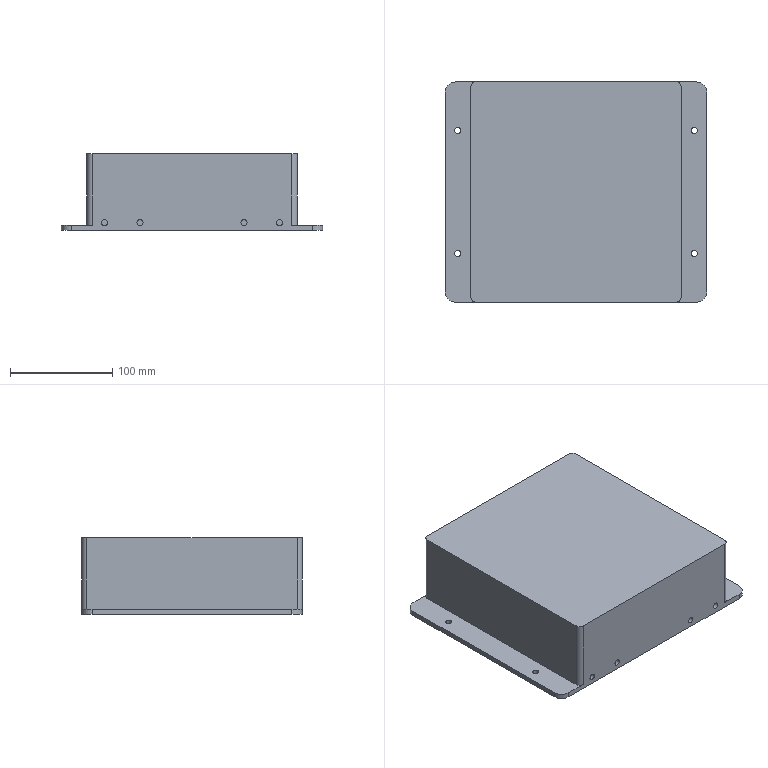NC program | NX | posted with a generic post | part box 255 x 215 x 75 mm
Lines 1 to 118 of 11258:
N10 G17 G21 G94 G90
(FLOOR_WALL_COPY , TOOL : D80)
N12 T19 M6
N14 G54
N16 G17 G0 G90 X-175.5 Y112.497 B0. C0. S6500 M3
N18 G43 Z30. H19
N20 Z7.
N22 G94 G1 Z4. F1500.
N24 X-172.5
N26 X172.5
N28 Y64.248
N30 X-172.5
N32 Y15.999
N34 X172.5
N36 Y-32.251
N38 X-172.5
N40 Y-80.5
N42 X172.5
N44 X175.5
N46 Z7.
N48 G0 Z30.
N50 X-175.5 Y112.497
N52 Z6.
N54 G1 Z3.
N56 X-172.5
N58 X172.5
N60 Y64.248
N62 X-172.5
N64 Y15.999
N66 X172.5
N68 Y-32.251
N70 X-172.5
N72 Y-80.5
N74 X172.5
N76 X175.5
N78 Z6.
N80 G0 Z30.
N82 X-175.5 Y112.497
N84 Z5.
N86 G1 Z2.
N88 X-172.5
N90 X172.5
N92 Y64.248
N94 X-172.5
N96 Y15.999
N98 X172.5
N100 Y-32.251
N102 X-172.5
N104 Y-80.5
N106 X172.5
N108 X175.5
N110 Z5.
N112 G0 Z30.
N114 X-175.5 Y112.497
N116 Z4.
N118 G1 Z1.
N120 X-172.5
N122 X172.5
N124 Y64.248
N126 X-172.5
N128 Y15.999
N130 X172.5
N132 Y-32.251
N134 X-172.5
N136 Y-80.5
N138 X172.5
N140 X175.5
N142 Z4.
N144 G0 Z30.
N146 X-175.5 Y112.497
N148 Z3.
N150 G1 Z0.
N152 X-172.5
N154 X172.5
N156 Y64.248
N158 X-172.5
N160 Y15.999
N162 X172.5
N164 Y-32.251
N166 X-172.5
N168 Y-80.5
N170 X172.5
N172 X175.5
N174 Z3.
N176 G0 Z30.
N178 M5
(DRILLING , TOOL : D6A45)
N180 T01 M6
N182 G54
N184 G17 G0 G90 X115.5 Y60. B0. C0. S5000 M3
N186 G43 Z30. H1
N188 G94 G81 G98 Z-1. F350. R3.
N190 Y-60.
N192 X-115.5
N194 Y60.
N196 G80
N198 G0 X-115.5 Y60. Z30.
N200 M5
(DRILLING_COPY , TOOL : 6.0ZT)
N202 T16 M6
N204 G54
N206 G17 G0 G90 X115.5 Y60. B0. C0. S2000 M3
N208 G43 Z30. H16
N210 G94 G83 G98 Z-8.303 F250. Q2. R3.
N212 Y-60.
N214 X-115.5
N216 Y60.
N218 G80
N220 G0 X-115.5 Y60. Z30.
N222 M5